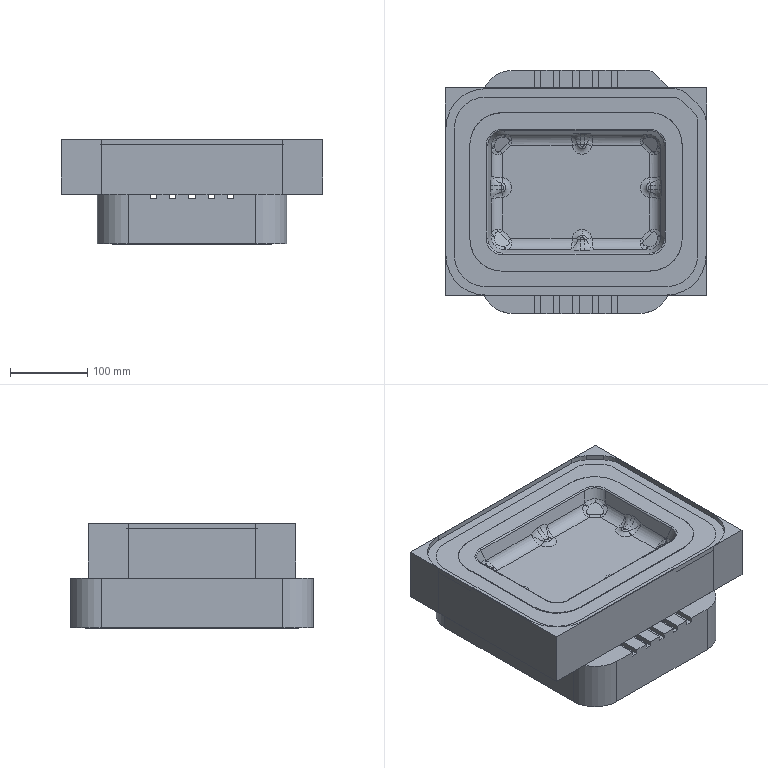NC program | NX | posted with a generic post | part box 339.125 x 315.125 x 135.5 mm
Lines 94177 to 94252 of 120728:
(DRILLING , TOOL : V2.0)
N188340 M6
N188342 G53
N188344 G17 G0 G90 X-84. Y50. S2000 M3 M8
N188346 G43 Z220.5 H0
N188348 G94 G81 G98 Z33.737 F150. R38.737
N188350 Y25.
N188352 Y0.
N188354 Y-25.
N188356 Y-50.
N188358 X-56.
N188360 Y-25.
N188362 Y0.
N188364 Y25.
N188366 Y50.
N188368 X-28.
N188370 Y25.
N188372 Y0.
N188374 Y-25.
N188376 Y-50.
N188378 X0.
N188380 X28.
N188382 Y-25.
N188384 X0.
N188386 Y0.
N188388 Y25.
N188390 Y50.
N188392 X28.
N188394 Y25.
N188396 Y0.
N188398 X56.
N188400 Y-25.
N188402 Y-50.
N188404 X84.
N188406 Y-25.
N188408 Y0.
N188410 Y25.
N188412 X56.
N188414 Y50.
N188416 X84.
N188418 X90.93 Y85.436 Z63. R68.
N188420 X114.278 Y76.512
N188422 X120.313 Y51.96
N188424 Y25.98
N188426 Y0.
N188428 Y-25.98
N188430 Y-51.96
N188432 X114.279 Y-76.511
N188434 X90.93 Y-85.436
N188436 X64.95
N188438 X38.97
N188440 X12.99
N188442 X-12.99
N188444 X-38.97
N188446 X-64.95
N188448 X-90.93
N188450 X-114.278 Y-76.512
N188452 X-120.313 Y-51.96
N188454 Y-25.98
N188456 Y0.
N188458 Y25.98
N188460 Y51.96
N188462 X-114.279 Y76.511
N188464 X-90.93 Y85.436
N188466 X-64.95
N188468 X-38.97
N188470 X-12.99
N188472 X12.99
N188474 X38.97
N188476 X64.95
N188478 G80
N188480 G0 X64.95 Y85.436 Z220.5
N188482 M9
N188484 M5